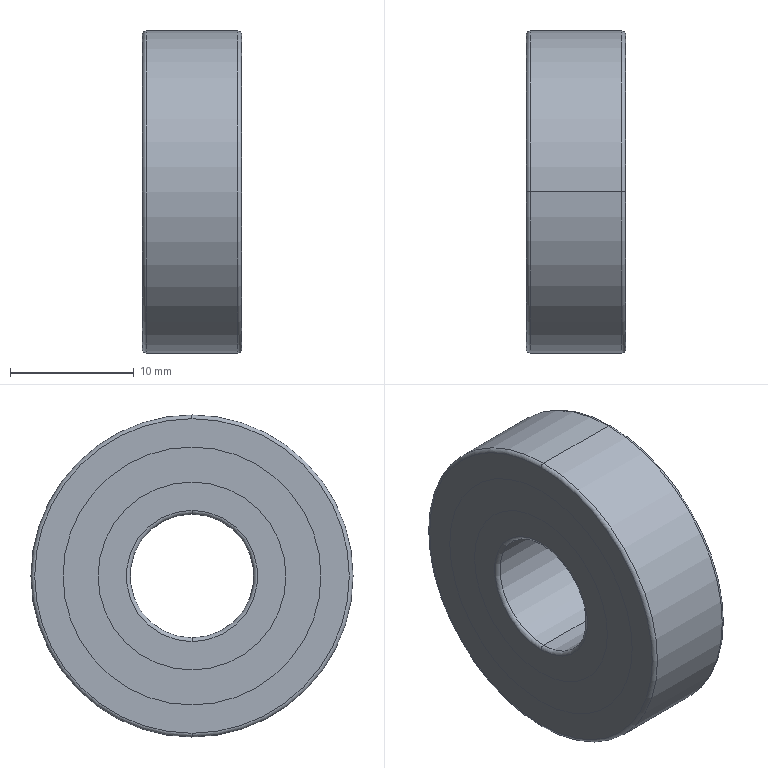Part | STEP file | 6000ZZ series deep groove ball bearing_6000ZZ | 5 solids | 46 faces | box 8 x 26 x 26 mm | volume 3330 mm3 | cylinder 20 | torus 18 | plane 8 | commonest cylinder face diameters 15.172 x8 20.828 x8 10 x2 26 x2